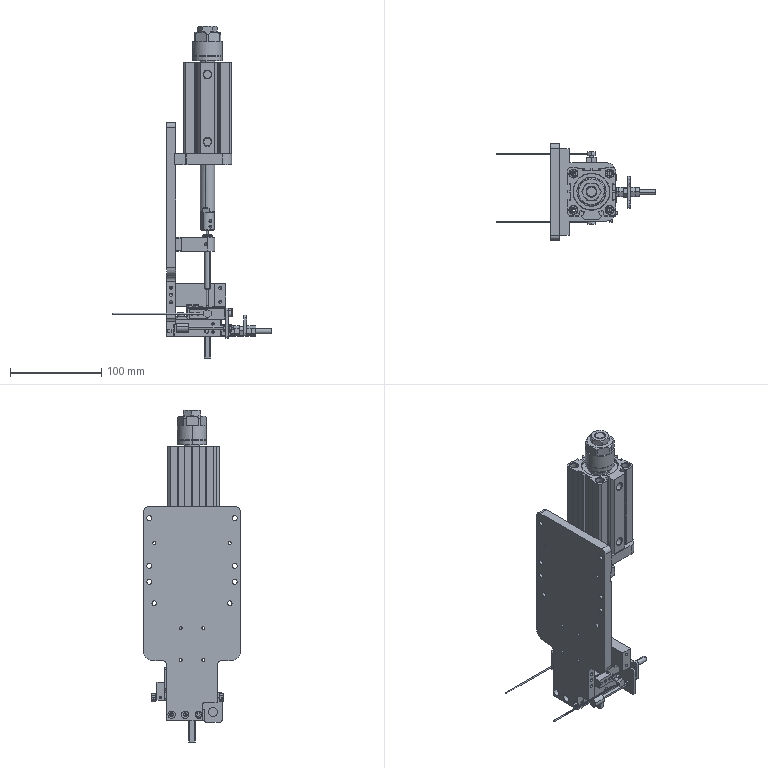Part | SolidWorks | features InContextFeatHolder 16 | 47 solids | 1396 faces | box 174 x 106 x 364.833 mm | volume 559956 mm3 | plane 592 | cylinder 555 | cone 211 | torus 32 | spline 6 | commonest cylinder face diameters 3.3 x72 4 x54 6 x40 2.5 x36 0.4 x35 3 x26